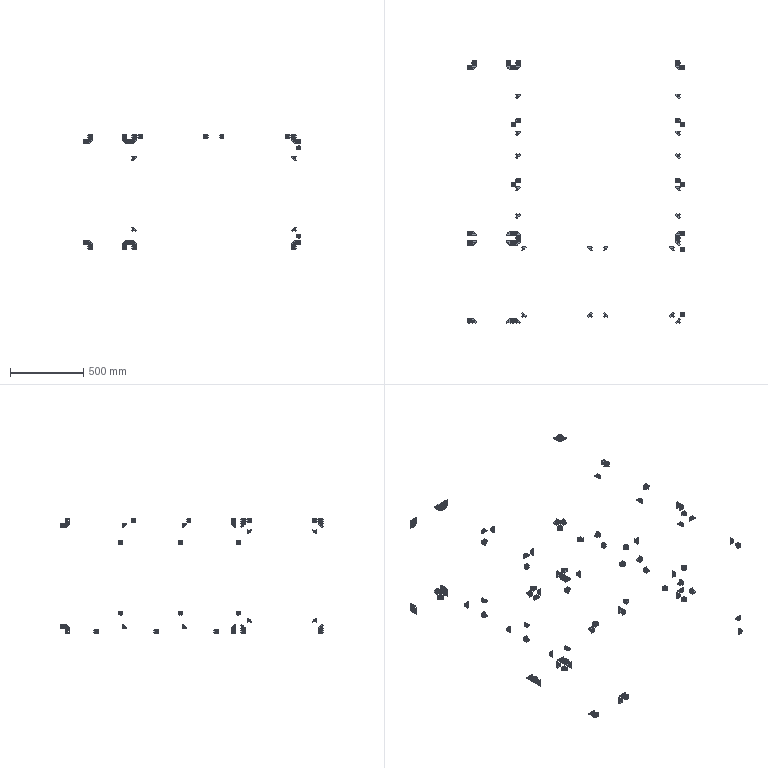Part | SolidWorks | 100 solids | 9500 faces | volume 806257 mm3 | plane 8600 | cylinder 900 | commonest cylinder face diameters 2 x700 2.5 x200